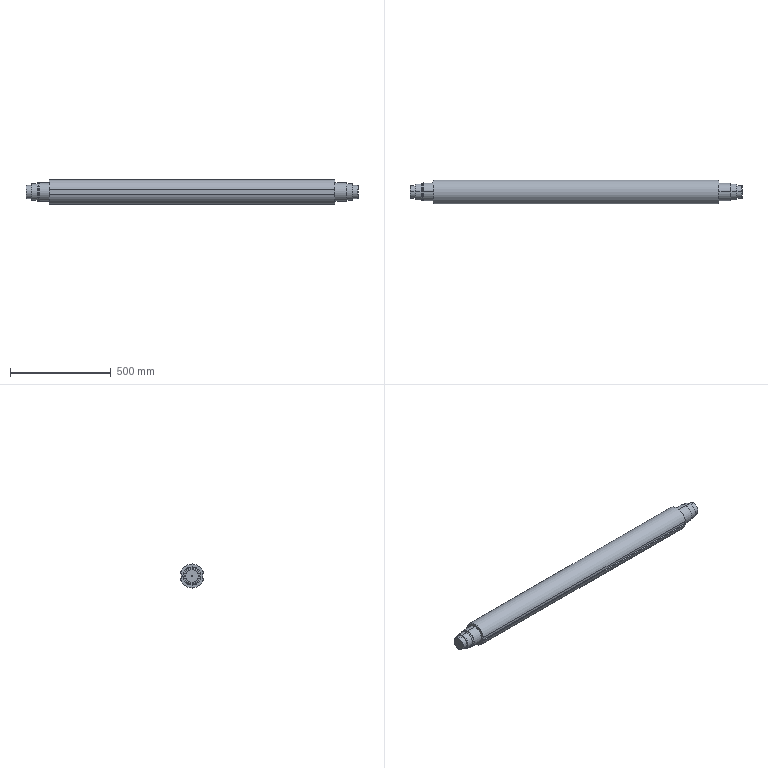Part | SolidWorks | features BaseBody 1 | 1 solid | 66 faces | box 1650 x 118.322 x 120 mm | volume 16871280 mm3 | cylinder 25 | cone 22 | plane 19 | commonest cylinder face diameters 90 x6 6 x4 65 x4 80 x4 120 x3 20 x2